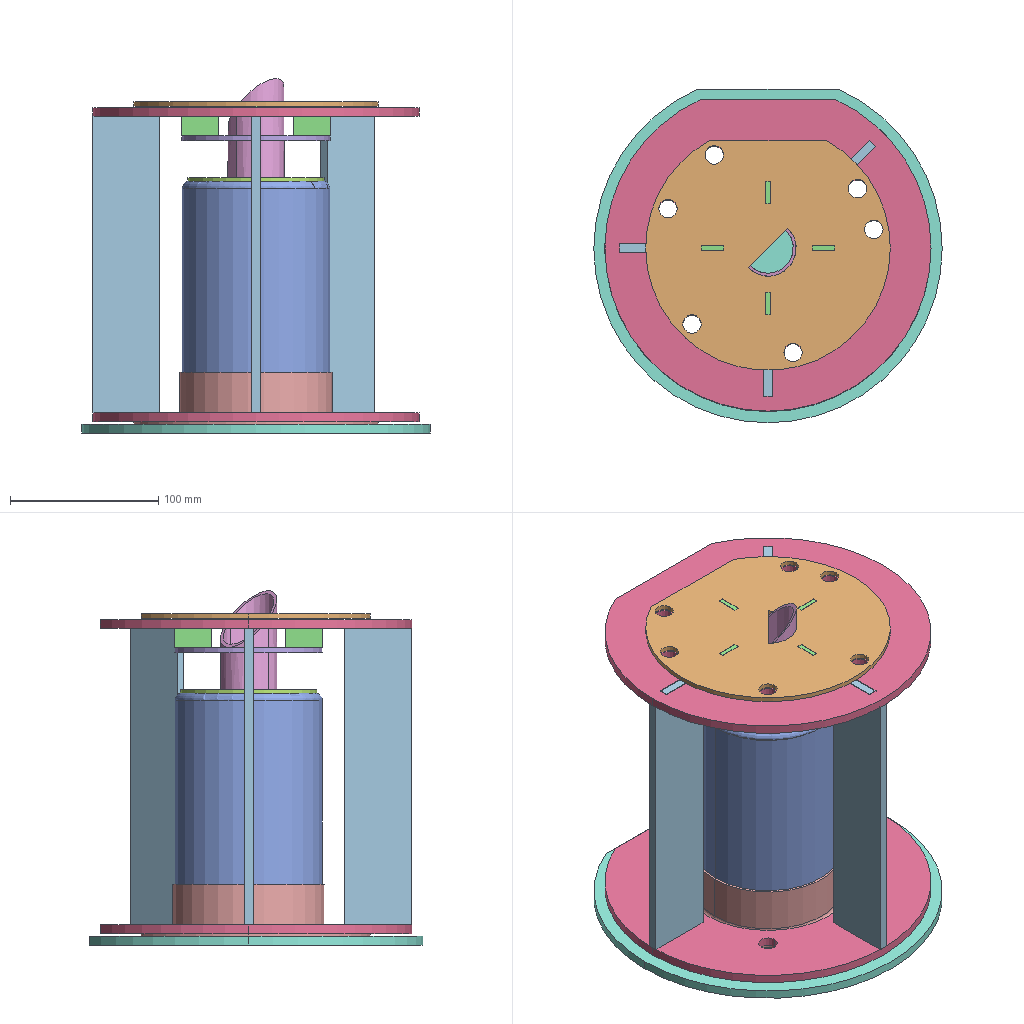Assembly | SolidWorks | 10 different items | 16 placed | box 235 x 225 x 239 mm
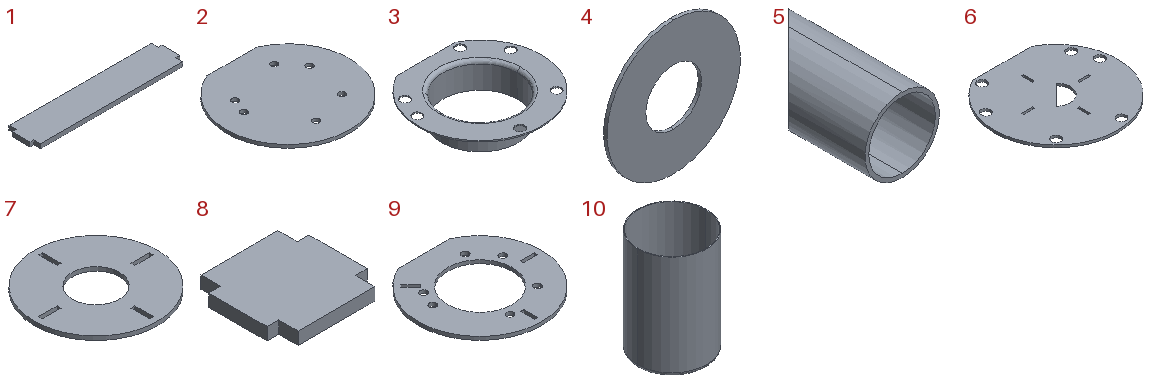Parts list (item | quantity | size | volume | features):
1 | x3 | 211 x 45 x 6 mm | 55650 mm3 | features Extrusion 1
2 | x1 | 235 x 225 x 6 mm | 251996 mm3 | features FlatPattern 1, SMBaseFlange 1, SheetMetal 1
3 | x1 | 165 x 155 x 35 mm | 35887 mm3 | features ICE 2, CirPattern 1, Fillet 1, RevolutionThin 1
4 | x1 | 92 x 2.3 x 92 mm | 12612 mm3 | features FlatPattern 1, SMBaseFlange 1, SheetMetal 1
5 | x1 | 38.1 x 77 x 38.1 mm | 13144 mm3 | features Extrusion 1, ICE 1
6 | x1 | 165 x 155 x 3.2 mm | 61928 mm3 | features FlatPattern 1, SMBaseFlange 1, SheetMetal 1
7 | x1 | 100 x 100 x 3.2 mm | 20870 mm3 | features FlatPattern 1, SMBaseFlange 1, SheetMetal 1
8 | x4 | 25.8 x 25 x 3.2 mm | 1872 mm3 | features Extrusion 1
9 | x2 | 220 x 210 x 6 mm | 154940 mm3 | features FlatPattern 1, SMBaseFlange 1, SheetMetal 1
10 | x1 | 99.6 x 99.6 x 150 mm | 51214 mm3 | features RevolutionThin 1
Mates (type | each side: item.copy, entity, surface, feature):
Concentric | 3.1 face cylinder Revolve-Thin2 | 10.1 face cylinder Revolve-Thin1
DistanceDim | 3.1 face plane Revolve-Thin2 | 10.1 face plane Revolve-Thin1
Coincident | 10.1 face plane Revolve-Thin1 | 4.1 face plane Base-Flange1
Concentric | 10.1 face cylinder Revolve-Thin1 | 4.1 face cylinder Base-Flange1
Coincident | 3.1 plane | 10.1 plane
Parallel | 4.1 plane | assembly plane
Concentric | 4.1 face cylinder Base-Flange1 | 5.1 face cylinder Boss-Extrude1
DistanceDim | 10.1 face plane Revolve-Thin1 | 5.1 face plane Boss-Extrude1
PlanarAngleDim | assembly plane | 5.1 plane
InPlace | 3.1 face plane Revolve-Thin2 | 2.1 plane
InPlace | 6.1 plane | assembly plane
InPlace | 7.1 plane | assembly plane
InPlace | 10.1 plane | 8.1 plane
InPlace | 9.1 plane | assembly plane
InPlace | 10.1 plane | 1.1 plane